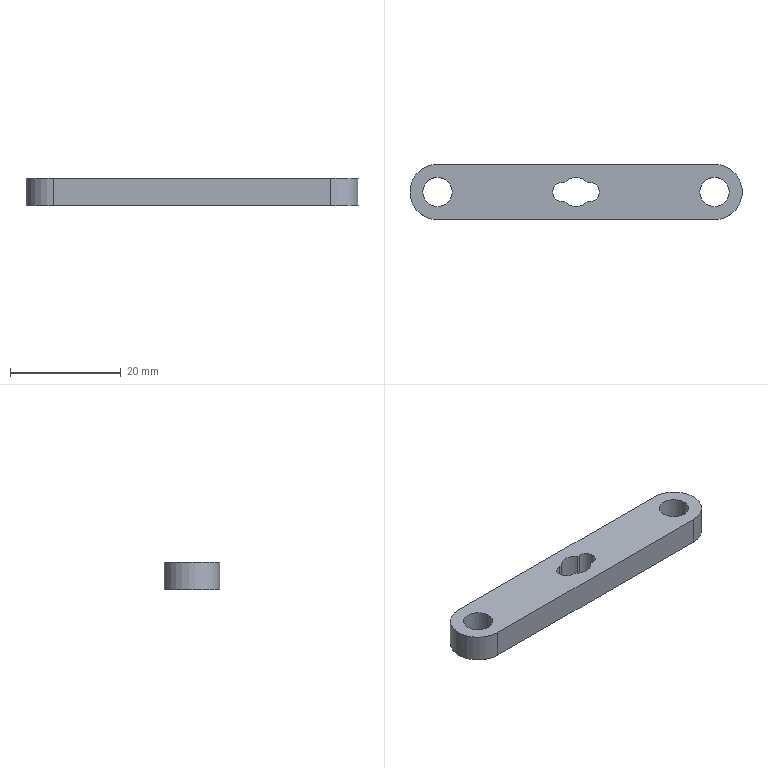Part | NX | features BREP 1 | 1 solid | 16 faces | box 60 x 10 x 5 mm | volume 2515 mm3 | cylinder 8 | plane 8 | commonest cylinder face diameters 5.3 x4 3.4 x2 10 x2
STEP:
#1=CARTESIAN_POINT('',(2.5,-1.7,-2.5));
#2=VERTEX_POINT('',#1);
#3=CARTESIAN_POINT('',(2.5,1.7,-2.5));
#4=VERTEX_POINT('',#3);
#5=CARTESIAN_POINT('',(2.5,0.,-2.5));
#6=DIRECTION('',(0.,0.,1.));
#7=DIRECTION('',(1.,0.,0.));
#8=AXIS2_PLACEMENT_3D('',#5,#6,#7);
#9=CIRCLE('',#8,1.7);
#10=EDGE_CURVE('',#2,#4,#9,.T.);
#11=ORIENTED_EDGE('',*,*,#10,.F.);
#12=CARTESIAN_POINT('',(2.5,-1.7,2.5));
#13=VERTEX_POINT('',#12);
#14=CARTESIAN_POINT('',(2.5,-1.7,-2.5));
#15=DIRECTION('',(0.,0.,1.));
#16=VECTOR('',#15,1000.);
#17=LINE('',#14,#16);
#18=EDGE_CURVE('',#2,#13,#17,.T.);
#19=ORIENTED_EDGE('',*,*,#18,.T.);
#20=CARTESIAN_POINT('',(2.5,1.7,2.5));
#21=VERTEX_POINT('',#20);
#22=CARTESIAN_POINT('',(2.5,0.,2.5));
#23=DIRECTION('',(0.,0.,1.));
#24=DIRECTION('',(1.,0.,0.));
#25=AXIS2_PLACEMENT_3D('',#22,#23,#24);
#26=CIRCLE('',#25,1.7);
#27=EDGE_CURVE('',#13,#21,#26,.T.);
#28=ORIENTED_EDGE('',*,*,#27,.T.);
#29=CARTESIAN_POINT('',(2.5,1.7,-2.5));
#30=DIRECTION('',(0.,0.,1.));
#31=VECTOR('',#30,1000.);
#32=LINE('',#29,#31);
#33=EDGE_CURVE('',#4,#21,#32,.T.);
#34=ORIENTED_EDGE('',*,*,#33,.F.);
#35=EDGE_LOOP('',(#11,#19,#28,#34));
#36=FACE_BOUND('',#35,.T.);
#37=CARTESIAN_POINT('',(2.5,0.,-2.5));
#38=DIRECTION('',(0.,0.,1.));
#39=DIRECTION('',(-1.,0.,0.));
#40=AXIS2_PLACEMENT_3D('',#37,#38,#39);
#41=CYLINDRICAL_SURFACE('',#40,1.7);
#42=ADVANCED_FACE('',(#36),#41,.F.);
#43=CARTESIAN_POINT('',(27.65,0.,2.5));
#44=VERTEX_POINT('',#43);
#45=CARTESIAN_POINT('',(25.,0.,2.5));
#46=DIRECTION('',(0.,0.,1.));
#47=DIRECTION('',(1.,0.,0.));
#48=AXIS2_PLACEMENT_3D('',#45,#46,#47);
#49=CIRCLE('',#48,2.65);
#50=EDGE_CURVE('',#44,#44,#49,.T.);
#51=ORIENTED_EDGE('',*,*,#50,.T.);
#52=EDGE_LOOP('',(#51));
#53=FACE_BOUND('',#52,.T.);
#54=CARTESIAN_POINT('',(27.65,0.,-2.5));
#55=VERTEX_POINT('',#54);
#56=CARTESIAN_POINT('',(25.,0.,-2.5));
#57=DIRECTION('',(0.,0.,1.));
#58=DIRECTION('',(1.,0.,0.));
#59=AXIS2_PLACEMENT_3D('',#56,#57,#58);
#60=CIRCLE('',#59,2.65);
#61=EDGE_CURVE('',#55,#55,#60,.T.);
#62=ORIENTED_EDGE('',*,*,#61,.F.);
#63=EDGE_LOOP('',(#62));
#64=FACE_BOUND('',#63,.T.);
#65=CARTESIAN_POINT('',(25.,0.,-2.5));
#66=DIRECTION('',(0.,0.,1.));
#67=DIRECTION('',(-1.,0.,0.));
#68=AXIS2_PLACEMENT_3D('',#65,#66,#67);
#69=CYLINDRICAL_SURFACE('',#68,2.65);
#70=ADVANCED_FACE('',(#53,#64),#69,.F.);
#71=CARTESIAN_POINT('',(-22.35,0.,2.5));
#72=VERTEX_POINT('',#71);
#73=CARTESIAN_POINT('',(-25.,0.,2.5));
#74=DIRECTION('',(0.,0.,1.));
#75=DIRECTION('',(1.,0.,0.));
#76=AXIS2_PLACEMENT_3D('',#73,#74,#75);
#77=CIRCLE('',#76,2.65);
#78=EDGE_CURVE('',#72,#72,#77,.T.);
#79=ORIENTED_EDGE('',*,*,#78,.T.);
#80=EDGE_LOOP('',(#79));
#81=FACE_BOUND('',#80,.T.);
#82=CARTESIAN_POINT('',(-22.35,0.,-2.5));
#83=VERTEX_POINT('',#82);
#84=CARTESIAN_POINT('',(-25.,0.,-2.5));
#85=DIRECTION('',(0.,0.,1.));
#86=DIRECTION('',(1.,0.,0.));
#87=AXIS2_PLACEMENT_3D('',#84,#85,#86);
#88=CIRCLE('',#87,2.65);
#89=EDGE_CURVE('',#83,#83,#88,.T.);
#90=ORIENTED_EDGE('',*,*,#89,.F.);
#91=EDGE_LOOP('',(#90));
#92=FACE_BOUND('',#91,.T.);
#93=CARTESIAN_POINT('',(-25.,0.,-2.5));
#94=DIRECTION('',(0.,0.,1.));
#95=DIRECTION('',(-1.,0.,0.));
#96=AXIS2_PLACEMENT_3D('',#93,#94,#95);
#97=CYLINDRICAL_SURFACE('',#96,2.65);
#98=ADVANCED_FACE('',(#81,#92),#97,.F.);
#99=CARTESIAN_POINT('',(-25.,5.,2.5));
#100=VERTEX_POINT('',#99);
#101=CARTESIAN_POINT('',(-25.,-5.,2.5));
#102=VERTEX_POINT('',#101);
#103=CARTESIAN_POINT('',(-25.,0.,2.5));
#104=DIRECTION('',(0.,0.,1.));
#105=DIRECTION('',(1.,0.,0.));
#106=AXIS2_PLACEMENT_3D('',#103,#104,#105);
#107=CIRCLE('',#106,5.);
#108=EDGE_CURVE('',#100,#102,#107,.T.);
#109=ORIENTED_EDGE('',*,*,#108,.F.);
#110=CARTESIAN_POINT('',(-25.,5.,-2.5));
#111=VERTEX_POINT('',#110);
#112=CARTESIAN_POINT('',(-25.,5.,2.5));
#113=DIRECTION('',(0.,0.,-1.));
#114=VECTOR('',#113,1000.);
#115=LINE('',#112,#114);
#116=EDGE_CURVE('',#100,#111,#115,.T.);
#117=ORIENTED_EDGE('',*,*,#116,.T.);
#118=CARTESIAN_POINT('',(-25.,-5.,-2.5));
#119=VERTEX_POINT('',#118);
#120=CARTESIAN_POINT('',(-25.,0.,-2.5));
#121=DIRECTION('',(0.,0.,1.));
#122=DIRECTION('',(1.,0.,0.));
#123=AXIS2_PLACEMENT_3D('',#120,#121,#122);
#124=CIRCLE('',#123,5.);
#125=EDGE_CURVE('',#111,#119,#124,.T.);
#126=ORIENTED_EDGE('',*,*,#125,.T.);
#127=CARTESIAN_POINT('',(-25.,-5.,2.5));
#128=DIRECTION('',(0.,0.,-1.));
#129=VECTOR('',#128,1000.);
#130=LINE('',#127,#129);
#131=EDGE_CURVE('',#102,#119,#130,.T.);
#132=ORIENTED_EDGE('',*,*,#131,.F.);
#133=EDGE_LOOP('',(#109,#117,#126,#132));
#134=FACE_BOUND('',#133,.T.);
#135=CARTESIAN_POINT('',(-25.,0.,2.5));
#136=DIRECTION('',(0.,0.,-1.));
#137=DIRECTION('',(1.,0.,0.));
#138=AXIS2_PLACEMENT_3D('',#135,#136,#137);
#139=CYLINDRICAL_SURFACE('',#138,5.);
#140=ADVANCED_FACE('',(#134),#139,.T.);
#141=CARTESIAN_POINT('',(2.033,1.7,2.5));
#142=VERTEX_POINT('',#141);
#143=CARTESIAN_POINT('',(-2.033,1.7,2.5));
#144=VERTEX_POINT('',#143);
#145=CARTESIAN_POINT('',(0.,0.,2.5));
#146=DIRECTION('',(0.,0.,1.));
#147=DIRECTION('',(1.,0.,0.));
#148=AXIS2_PLACEMENT_3D('',#145,#146,#147);
#149=CIRCLE('',#148,2.65);
#150=EDGE_CURVE('',#142,#144,#149,.T.);
#151=ORIENTED_EDGE('',*,*,#150,.T.);
#152=CARTESIAN_POINT('',(-2.033,1.7,-2.5));
#153=VERTEX_POINT('',#152);
#154=CARTESIAN_POINT('',(-2.033,1.7,-2.5));
#155=DIRECTION('',(0.,0.,-1.));
#156=VECTOR('',#155,1000.);
#157=LINE('',#154,#156);
#158=EDGE_CURVE('',#144,#153,#157,.T.);
#159=ORIENTED_EDGE('',*,*,#158,.T.);
#160=CARTESIAN_POINT('',(2.033,1.7,-2.5));
#161=VERTEX_POINT('',#160);
#162=CARTESIAN_POINT('',(0.,0.,-2.5));
#163=DIRECTION('',(0.,0.,1.));
#164=DIRECTION('',(1.,0.,0.));
#165=AXIS2_PLACEMENT_3D('',#162,#163,#164);
#166=CIRCLE('',#165,2.65);
#167=EDGE_CURVE('',#161,#153,#166,.T.);
#168=ORIENTED_EDGE('',*,*,#167,.F.);
#169=CARTESIAN_POINT('',(2.033,1.7,-2.5));
#170=DIRECTION('',(0.,0.,1.));
#171=VECTOR('',#170,1000.);
#172=LINE('',#169,#171);
#173=EDGE_CURVE('',#161,#142,#172,.T.);
#174=ORIENTED_EDGE('',*,*,#173,.T.);
#175=EDGE_LOOP('',(#151,#159,#168,#174));
#176=FACE_BOUND('',#175,.T.);
#177=CARTESIAN_POINT('',(0.,0.,-2.5));
#178=DIRECTION('',(0.,0.,1.));
#179=DIRECTION('',(-1.,0.,0.));
#180=AXIS2_PLACEMENT_3D('',#177,#178,#179);
#181=CYLINDRICAL_SURFACE('',#180,2.65);
#182=ADVANCED_FACE('',(#176),#181,.F.);
#183=CARTESIAN_POINT('',(25.,-5.,-2.5));
#184=VERTEX_POINT('',#183);
#185=CARTESIAN_POINT('',(-25.,-5.,-2.5));
#186=DIRECTION('',(1.,0.,0.));
#187=VECTOR('',#186,1000.);
#188=LINE('',#185,#187);
#189=EDGE_CURVE('',#119,#184,#188,.T.);
#190=ORIENTED_EDGE('',*,*,#189,.T.);
#191=CARTESIAN_POINT('',(25.,-5.,2.5));
#192=VERTEX_POINT('',#191);
#193=CARTESIAN_POINT('',(25.,-5.,2.5));
#194=DIRECTION('',(0.,0.,-1.));
#195=VECTOR('',#194,1000.);
#196=LINE('',#193,#195);
#197=EDGE_CURVE('',#192,#184,#196,.T.);
#198=ORIENTED_EDGE('',*,*,#197,.F.);
#199=CARTESIAN_POINT('',(-25.,-5.,2.5));
#200=DIRECTION('',(1.,0.,0.));
#201=VECTOR('',#200,1000.);
#202=LINE('',#199,#201);
#203=EDGE_CURVE('',#102,#192,#202,.T.);
#204=ORIENTED_EDGE('',*,*,#203,.F.);
#205=ORIENTED_EDGE('',*,*,#131,.T.);
#206=EDGE_LOOP('',(#190,#198,#204,#205));
#207=FACE_BOUND('',#206,.T.);
#208=CARTESIAN_POINT('',(-25.,-5.,2.5));
#209=DIRECTION('',(0.,1.,0.));
#210=DIRECTION('',(0.,0.,-1.));
#211=AXIS2_PLACEMENT_3D('',#208,#209,#210);
#212=PLANE('',#211);
#213=ADVANCED_FACE('',(#207),#212,.F.);
#214=CARTESIAN_POINT('',(25.,5.,-2.5));
#215=VERTEX_POINT('',#214);
#216=CARTESIAN_POINT('',(25.,0.,-2.5));
#217=DIRECTION('',(0.,0.,1.));
#218=DIRECTION('',(1.,0.,0.));
#219=AXIS2_PLACEMENT_3D('',#216,#217,#218);
#220=CIRCLE('',#219,5.);
#221=EDGE_CURVE('',#184,#215,#220,.T.);
#222=ORIENTED_EDGE('',*,*,#221,.T.);
#223=CARTESIAN_POINT('',(25.,5.,2.5));
#224=VERTEX_POINT('',#223);
#225=CARTESIAN_POINT('',(25.,5.,2.5));
#226=DIRECTION('',(0.,0.,-1.));
#227=VECTOR('',#226,1000.);
#228=LINE('',#225,#227);
#229=EDGE_CURVE('',#224,#215,#228,.T.);
#230=ORIENTED_EDGE('',*,*,#229,.F.);
#231=CARTESIAN_POINT('',(25.,0.,2.5));
#232=DIRECTION('',(0.,0.,1.));
#233=DIRECTION('',(1.,0.,0.));
#234=AXIS2_PLACEMENT_3D('',#231,#232,#233);
#235=CIRCLE('',#234,5.);
#236=EDGE_CURVE('',#192,#224,#235,.T.);
#237=ORIENTED_EDGE('',*,*,#236,.F.);
#238=ORIENTED_EDGE('',*,*,#197,.T.);
#239=EDGE_LOOP('',(#222,#230,#237,#238));
#240=FACE_BOUND('',#239,.T.);
#241=CARTESIAN_POINT('',(25.,0.,2.5));
#242=DIRECTION('',(0.,0.,-1.));
#243=DIRECTION('',(1.,0.,0.));
#244=AXIS2_PLACEMENT_3D('',#241,#242,#243);
#245=CYLINDRICAL_SURFACE('',#244,5.);
#246=ADVANCED_FACE('',(#240),#245,.T.);
#247=CARTESIAN_POINT('',(-25.,5.,-2.5));
#248=DIRECTION('',(-1.,0.,0.));
#249=VECTOR('',#248,1000.);
#250=LINE('',#247,#249);
#251=EDGE_CURVE('',#215,#111,#250,.T.);
#252=ORIENTED_EDGE('',*,*,#251,.T.);
#253=ORIENTED_EDGE('',*,*,#116,.F.);
#254=CARTESIAN_POINT('',(-25.,5.,2.5));
#255=DIRECTION('',(-1.,0.,0.));
#256=VECTOR('',#255,1000.);
#257=LINE('',#254,#256);
#258=EDGE_CURVE('',#224,#100,#257,.T.);
#259=ORIENTED_EDGE('',*,*,#258,.F.);
#260=ORIENTED_EDGE('',*,*,#229,.T.);
#261=EDGE_LOOP('',(#252,#253,#259,#260));
#262=FACE_BOUND('',#261,.T.);
#263=CARTESIAN_POINT('',(-25.,5.,2.5));
#264=DIRECTION('',(0.,-1.,0.));
#265=DIRECTION('',(-1.,0.,0.));
#266=AXIS2_PLACEMENT_3D('',#263,#264,#265);
#267=PLANE('',#266);
#268=ADVANCED_FACE('',(#262),#267,.F.);
#269=CARTESIAN_POINT('',(-2.5,1.7,2.5));
#270=VERTEX_POINT('',#269);
#271=CARTESIAN_POINT('',(-2.5,1.7,2.5));
#272=DIRECTION('',(-1.,0.,0.));
#273=VECTOR('',#272,1000.);
#274=LINE('',#271,#273);
#275=EDGE_CURVE('',#144,#270,#274,.T.);
#276=ORIENTED_EDGE('',*,*,#275,.F.);
#277=ORIENTED_EDGE('',*,*,#150,.F.);
#278=CARTESIAN_POINT('',(-2.5,1.7,2.5));
#279=DIRECTION('',(-1.,0.,0.));
#280=VECTOR('',#279,1000.);
#281=LINE('',#278,#280);
#282=EDGE_CURVE('',#21,#142,#281,.T.);
#283=ORIENTED_EDGE('',*,*,#282,.F.);
#284=ORIENTED_EDGE('',*,*,#27,.F.);
#285=CARTESIAN_POINT('',(2.033,-1.7,2.5));
#286=VERTEX_POINT('',#285);
#287=CARTESIAN_POINT('',(-2.5,-1.7,2.5));
#288=DIRECTION('',(1.,0.,0.));
#289=VECTOR('',#288,1000.);
#290=LINE('',#287,#289);
#291=EDGE_CURVE('',#286,#13,#290,.T.);
#292=ORIENTED_EDGE('',*,*,#291,.F.);
#293=CARTESIAN_POINT('',(-2.033,-1.7,2.5));
#294=VERTEX_POINT('',#293);
#295=CARTESIAN_POINT('',(0.,0.,2.5));
#296=DIRECTION('',(0.,0.,1.));
#297=DIRECTION('',(1.,0.,0.));
#298=AXIS2_PLACEMENT_3D('',#295,#296,#297);
#299=CIRCLE('',#298,2.65);
#300=EDGE_CURVE('',#294,#286,#299,.T.);
#301=ORIENTED_EDGE('',*,*,#300,.F.);
#302=CARTESIAN_POINT('',(-2.5,-1.7,2.5));
#303=VERTEX_POINT('',#302);
#304=CARTESIAN_POINT('',(-2.5,-1.7,2.5));
#305=DIRECTION('',(1.,0.,0.));
#306=VECTOR('',#305,1000.);
#307=LINE('',#304,#306);
#308=EDGE_CURVE('',#303,#294,#307,.T.);
#309=ORIENTED_EDGE('',*,*,#308,.F.);
#310=CARTESIAN_POINT('',(-2.5,0.,2.5));
#311=DIRECTION('',(0.,0.,1.));
#312=DIRECTION('',(1.,0.,0.));
#313=AXIS2_PLACEMENT_3D('',#310,#311,#312);
#314=CIRCLE('',#313,1.7);
#315=EDGE_CURVE('',#270,#303,#314,.T.);
#316=ORIENTED_EDGE('',*,*,#315,.F.);
#317=EDGE_LOOP('',(#276,#277,#283,#284,#292,#301,#309,#316));
#318=FACE_BOUND('',#317,.T.);
#319=ORIENTED_EDGE('',*,*,#50,.F.);
#320=EDGE_LOOP('',(#319));
#321=FACE_BOUND('',#320,.T.);
#322=ORIENTED_EDGE('',*,*,#78,.F.);
#323=EDGE_LOOP('',(#322));
#324=FACE_BOUND('',#323,.T.);
#325=ORIENTED_EDGE('',*,*,#258,.T.);
#326=ORIENTED_EDGE('',*,*,#108,.T.);
#327=ORIENTED_EDGE('',*,*,#203,.T.);
#328=ORIENTED_EDGE('',*,*,#236,.T.);
#329=EDGE_LOOP('',(#325,#326,#327,#328));
#330=FACE_BOUND('',#329,.T.);
#331=CARTESIAN_POINT('',(-25.,0.,2.5));
#332=DIRECTION('',(0.,0.,1.));
#333=DIRECTION('',(-1.,0.,0.));
#334=AXIS2_PLACEMENT_3D('',#331,#332,#333);
#335=PLANE('',#334);
#336=ADVANCED_FACE('',(#318,#321,#324,#330),#335,.T.);
#337=ORIENTED_EDGE('',*,*,#167,.T.);
#338=CARTESIAN_POINT('',(-2.5,1.7,-2.5));
#339=VERTEX_POINT('',#338);
#340=CARTESIAN_POINT('',(-2.5,1.7,-2.5));
#341=DIRECTION('',(-1.,0.,0.));
#342=VECTOR('',#341,1000.);
#343=LINE('',#340,#342);
#344=EDGE_CURVE('',#153,#339,#343,.T.);
#345=ORIENTED_EDGE('',*,*,#344,.T.);
#346=CARTESIAN_POINT('',(-2.5,-1.7,-2.5));
#347=VERTEX_POINT('',#346);
#348=CARTESIAN_POINT('',(-2.5,0.,-2.5));
#349=DIRECTION('',(0.,0.,1.));
#350=DIRECTION('',(1.,0.,0.));
#351=AXIS2_PLACEMENT_3D('',#348,#349,#350);
#352=CIRCLE('',#351,1.7);
#353=EDGE_CURVE('',#339,#347,#352,.T.);
#354=ORIENTED_EDGE('',*,*,#353,.T.);
#355=CARTESIAN_POINT('',(-2.033,-1.7,-2.5));
#356=VERTEX_POINT('',#355);
#357=CARTESIAN_POINT('',(-2.5,-1.7,-2.5));
#358=DIRECTION('',(1.,0.,0.));
#359=VECTOR('',#358,1000.);
#360=LINE('',#357,#359);
#361=EDGE_CURVE('',#347,#356,#360,.T.);
#362=ORIENTED_EDGE('',*,*,#361,.T.);
#363=CARTESIAN_POINT('',(2.033,-1.7,-2.5));
#364=VERTEX_POINT('',#363);
#365=CARTESIAN_POINT('',(0.,0.,-2.5));
#366=DIRECTION('',(0.,0.,1.));
#367=DIRECTION('',(1.,0.,0.));
#368=AXIS2_PLACEMENT_3D('',#365,#366,#367);
#369=CIRCLE('',#368,2.65);
#370=EDGE_CURVE('',#356,#364,#369,.T.);
#371=ORIENTED_EDGE('',*,*,#370,.T.);
#372=CARTESIAN_POINT('',(-2.5,-1.7,-2.5));
#373=DIRECTION('',(1.,0.,0.));
#374=VECTOR('',#373,1000.);
#375=LINE('',#372,#374);
#376=EDGE_CURVE('',#364,#2,#375,.T.);
#377=ORIENTED_EDGE('',*,*,#376,.T.);
#378=ORIENTED_EDGE('',*,*,#10,.T.);
#379=CARTESIAN_POINT('',(-2.5,1.7,-2.5));
#380=DIRECTION('',(-1.,0.,0.));
#381=VECTOR('',#380,1000.);
#382=LINE('',#379,#381);
#383=EDGE_CURVE('',#4,#161,#382,.T.);
#384=ORIENTED_EDGE('',*,*,#383,.T.);
#385=EDGE_LOOP('',(#337,#345,#354,#362,#371,#377,#378,#384));
#386=FACE_BOUND('',#385,.T.);
#387=ORIENTED_EDGE('',*,*,#61,.T.);
#388=EDGE_LOOP('',(#387));
#389=FACE_BOUND('',#388,.T.);
#390=ORIENTED_EDGE('',*,*,#89,.T.);
#391=EDGE_LOOP('',(#390));
#392=FACE_BOUND('',#391,.T.);
#393=ORIENTED_EDGE('',*,*,#125,.F.);
#394=ORIENTED_EDGE('',*,*,#251,.F.);
#395=ORIENTED_EDGE('',*,*,#221,.F.);
#396=ORIENTED_EDGE('',*,*,#189,.F.);
#397=EDGE_LOOP('',(#393,#394,#395,#396));
#398=FACE_BOUND('',#397,.T.);
#399=CARTESIAN_POINT('',(-25.,0.,-2.5));
#400=DIRECTION('',(0.,0.,1.));
#401=DIRECTION('',(-1.,0.,0.));
#402=AXIS2_PLACEMENT_3D('',#399,#400,#401);
#403=PLANE('',#402);
#404=ADVANCED_FACE('',(#386,#389,#392,#398),#403,.F.);
#405=ORIENTED_EDGE('',*,*,#300,.T.);
#406=CARTESIAN_POINT('',(2.033,-1.7,-2.5));
#407=DIRECTION('',(0.,0.,-1.));
#408=VECTOR('',#407,1000.);
#409=LINE('',#406,#408);
#410=EDGE_CURVE('',#286,#364,#409,.T.);
#411=ORIENTED_EDGE('',*,*,#410,.T.);
#412=ORIENTED_EDGE('',*,*,#370,.F.);
#413=CARTESIAN_POINT('',(-2.033,-1.7,-2.5));
#414=DIRECTION('',(0.,0.,1.));
#415=VECTOR('',#414,1000.);
#416=LINE('',#413,#415);
#417=EDGE_CURVE('',#356,#294,#416,.T.);
#418=ORIENTED_EDGE('',*,*,#417,.T.);
#419=EDGE_LOOP('',(#405,#411,#412,#418));
#420=FACE_BOUND('',#419,.T.);
#421=CARTESIAN_POINT('',(0.,0.,-2.5));
#422=DIRECTION('',(0.,0.,1.));
#423=DIRECTION('',(-1.,0.,0.));
#424=AXIS2_PLACEMENT_3D('',#421,#422,#423);
#425=CYLINDRICAL_SURFACE('',#424,2.65);
#426=ADVANCED_FACE('',(#420),#425,.F.);
#427=ORIENTED_EDGE('',*,*,#361,.F.);
#428=CARTESIAN_POINT('',(-2.5,-1.7,-2.5));
#429=DIRECTION('',(0.,0.,1.));
#430=VECTOR('',#429,1000.);
#431=LINE('',#428,#430);
#432=EDGE_CURVE('',#347,#303,#431,.T.);
#433=ORIENTED_EDGE('',*,*,#432,.T.);
#434=ORIENTED_EDGE('',*,*,#308,.T.);
#435=ORIENTED_EDGE('',*,*,#417,.F.);
#436=EDGE_LOOP('',(#427,#433,#434,#435));
#437=FACE_BOUND('',#436,.T.);
#438=CARTESIAN_POINT('',(-2.5,-1.7,-2.5));
#439=DIRECTION('',(0.,-1.,0.));
#440=DIRECTION('',(0.,0.,1.));
#441=AXIS2_PLACEMENT_3D('',#438,#439,#440);
#442=PLANE('',#441);
#443=ADVANCED_FACE('',(#437),#442,.F.);
#444=ORIENTED_EDGE('',*,*,#275,.T.);
#445=CARTESIAN_POINT('',(-2.5,1.7,-2.5));
#446=DIRECTION('',(0.,0.,1.));
#447=VECTOR('',#446,1000.);
#448=LINE('',#445,#447);
#449=EDGE_CURVE('',#339,#270,#448,.T.);
#450=ORIENTED_EDGE('',*,*,#449,.F.);
#451=ORIENTED_EDGE('',*,*,#344,.F.);
#452=ORIENTED_EDGE('',*,*,#158,.F.);
#453=EDGE_LOOP('',(#444,#450,#451,#452));
#454=FACE_BOUND('',#453,.T.);
#455=CARTESIAN_POINT('',(-2.5,1.7,-2.5));
#456=DIRECTION('',(0.,1.,0.));
#457=DIRECTION('',(0.,0.,-1.));
#458=AXIS2_PLACEMENT_3D('',#455,#456,#457);
#459=PLANE('',#458);
#460=ADVANCED_FACE('',(#454),#459,.F.);
#461=ORIENTED_EDGE('',*,*,#315,.T.);
#462=ORIENTED_EDGE('',*,*,#432,.F.);
#463=ORIENTED_EDGE('',*,*,#353,.F.);
#464=ORIENTED_EDGE('',*,*,#449,.T.);
#465=EDGE_LOOP('',(#461,#462,#463,#464));
#466=FACE_BOUND('',#465,.T.);
#467=CARTESIAN_POINT('',(-2.5,0.,-2.5));
#468=DIRECTION('',(0.,0.,1.));
#469=DIRECTION('',(-1.,0.,0.));
#470=AXIS2_PLACEMENT_3D('',#467,#468,#469);
#471=CYLINDRICAL_SURFACE('',#470,1.7);
#472=ADVANCED_FACE('',(#466),#471,.F.);
#473=ORIENTED_EDGE('',*,*,#383,.F.);
#474=ORIENTED_EDGE('',*,*,#33,.T.);
#475=ORIENTED_EDGE('',*,*,#282,.T.);
#476=ORIENTED_EDGE('',*,*,#173,.F.);
#477=EDGE_LOOP('',(#473,#474,#475,#476));
#478=FACE_BOUND('',#477,.T.);
#479=CARTESIAN_POINT('',(-2.5,1.7,-2.5));
#480=DIRECTION('',(0.,1.,0.));
#481=DIRECTION('',(0.,0.,-1.));
#482=AXIS2_PLACEMENT_3D('',#479,#480,#481);
#483=PLANE('',#482);
#484=ADVANCED_FACE('',(#478),#483,.F.);
#485=ORIENTED_EDGE('',*,*,#291,.T.);
#486=ORIENTED_EDGE('',*,*,#18,.F.);
#487=ORIENTED_EDGE('',*,*,#376,.F.);
#488=ORIENTED_EDGE('',*,*,#410,.F.);
#489=EDGE_LOOP('',(#485,#486,#487,#488));
#490=FACE_BOUND('',#489,.T.);
#491=CARTESIAN_POINT('',(-2.5,-1.7,-2.5));
#492=DIRECTION('',(0.,-1.,0.));
#493=DIRECTION('',(0.,0.,1.));
#494=AXIS2_PLACEMENT_3D('',#491,#492,#493);
#495=PLANE('',#494);
#496=ADVANCED_FACE('',(#490),#495,.F.);
#497=CLOSED_SHELL('',(#42,#70,#98,#140,#182,#213,#246,#268,#336,#404,#426,#443,#460,#472,#484,#496));
#498=MANIFOLD_SOLID_BREP('',#497);
#499=(LENGTH_UNIT()NAMED_UNIT(*)SI_UNIT(.MILLI.,.METRE.));
#500=UNCERTAINTY_MEASURE_WITH_UNIT(LENGTH_MEASURE(0.00001),#499,'','');
#501=(NAMED_UNIT(*)PLANE_ANGLE_UNIT()SI_UNIT($,.RADIAN.));
#502=(NAMED_UNIT(*)SI_UNIT($,.STERADIAN.)SOLID_ANGLE_UNIT());
#503=(GEOMETRIC_REPRESENTATION_CONTEXT(3)GLOBAL_UNCERTAINTY_ASSIGNED_CONTEXT((#500))GLOBAL_UNIT_ASSIGNED_CONTEXT((#499,#501,#502))REPRESENTATION_CONTEXT('',''));
#504=ADVANCED_BREP_SHAPE_REPRESENTATION('',(#498),#503);